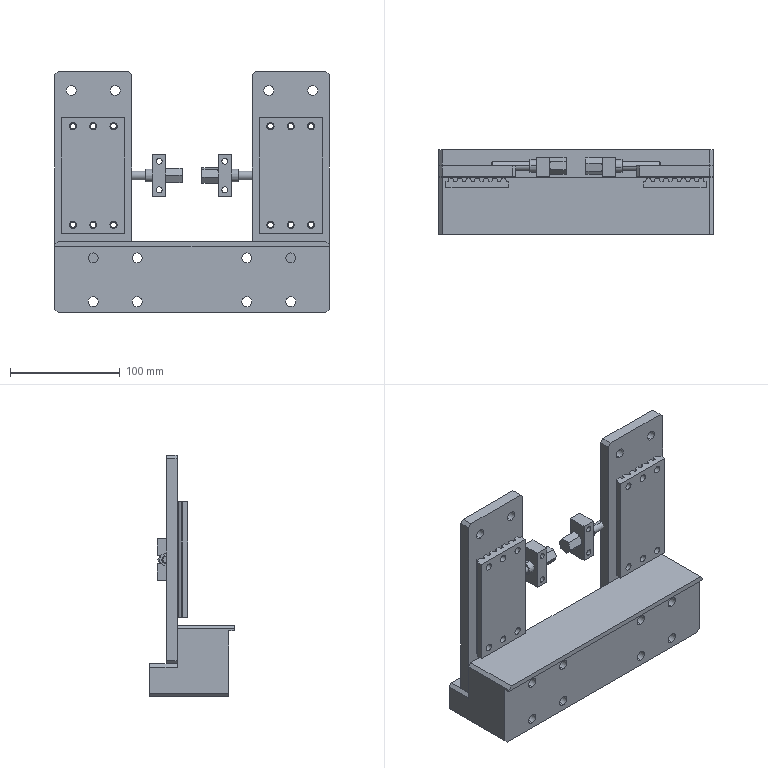Part | SolidWorks | 9 solids | 414 faces | box 250 x 77 x 220 mm | volume 1248427 mm3 | cylinder 236 | plane 140 | cone 38 | commonest cylinder face diameters 1.6 x44 10.4 x44 9 x32 5 x24 6.6 x24 6.8 x16